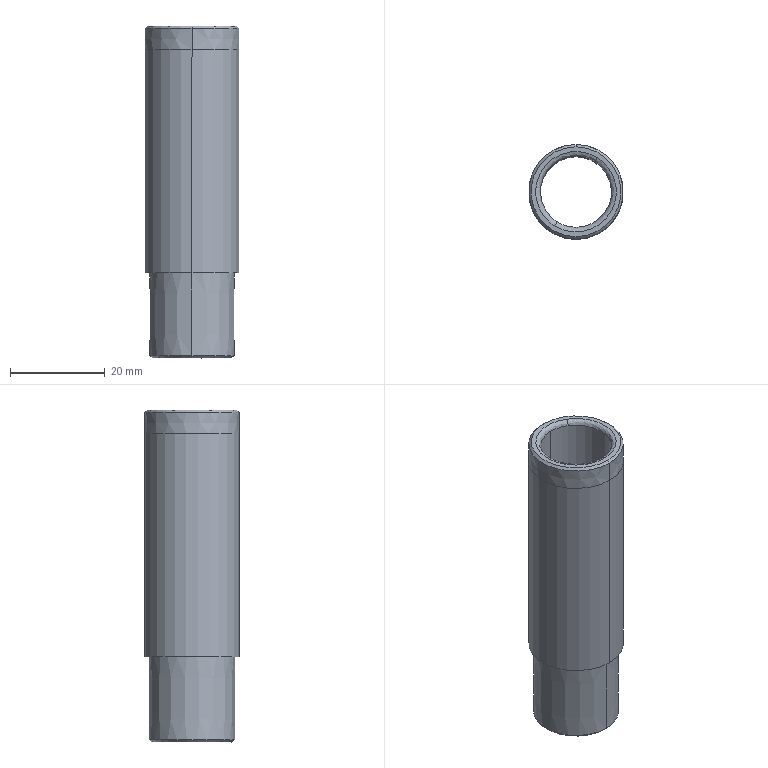Part | SolidWorks | features BaseBody 1 | 1 solid | 19 faces | box 20 x 20 x 70.171 mm | volume 8540 mm3 | cone 8 | spline 4 | cylinder 4 | plane 3 | commonest cylinder face diameters 15 x2 20 x2
STEP:
#1=CARTESIAN_POINT('',(700.535,31.172,-70.73));
#2=VERTEX_POINT('',#1);
#3=CARTESIAN_POINT('',(704.511,45.031,-70.73));
#4=VERTEX_POINT('',#3);
#5=CARTESIAN_POINT('',(700.535,38.672,-70.73));
#6=DIRECTION('',(0.000000001,-0.000000003,1.));
#7=DIRECTION('',(0.,-1.,-0.000000003));
#8=AXIS2_PLACEMENT_3D('',#5,#6,#7);
#9=CIRCLE('',#8,7.5);
#10=EDGE_CURVE('',#2,#4,#9,.T.);
#11=ORIENTED_EDGE('',*,*,#10,.T.);
#12=CARTESIAN_POINT('',(704.776,45.455,-71.23));
#13=VERTEX_POINT('',#12);
#14=CARTESIAN_POINT('',(704.776,45.455,-70.73));
#15=DIRECTION('',(0.8479,-0.5302,-0.000000002));
#16=DIRECTION('',(0.5302,0.8479,0.000000002));
#17=AXIS2_PLACEMENT_3D('',#14,#15,#16);
#18=CIRCLE('',#17,0.5);
#19=EDGE_CURVE('',#4,#13,#18,.T.);
#20=ORIENTED_EDGE('',*,*,#19,.T.);
#21=CARTESIAN_POINT('',(696.293,31.889,-71.23));
#22=VERTEX_POINT('',#21);
#23=CARTESIAN_POINT('',(704.776,45.455,-71.23));
#24=CARTESIAN_POINT('',(718.342,36.972,-71.23));
#25=CARTESIAN_POINT('',(709.86,23.406,-71.23));
#26=CARTESIAN_POINT('',(696.293,31.889,-71.23));
#27=(BOUNDED_CURVE()B_SPLINE_CURVE(3,(#23,#24,#25,#26),.UNSPECIFIED.,.F.,.F.)B_SPLINE_CURVE_WITH_KNOTS((4,4),(0.,1.),.UNSPECIFIED.)CURVE()GEOMETRIC_REPRESENTATION_ITEM()RATIONAL_B_SPLINE_CURVE((1.,0.3333,0.3333,1.))REPRESENTATION_ITEM(''));
#28=EDGE_CURVE('',#13,#22,#27,.T.);
#29=ORIENTED_EDGE('',*,*,#28,.T.);
#30=CARTESIAN_POINT('',(696.558,32.313,-70.73));
#31=VERTEX_POINT('',#30);
#32=CARTESIAN_POINT('',(696.293,31.889,-70.73));
#33=DIRECTION('',(-0.8479,0.5302,0.000000002));
#34=DIRECTION('',(-0.5302,-0.8479,-0.000000002));
#35=AXIS2_PLACEMENT_3D('',#32,#33,#34);
#36=CIRCLE('',#35,0.5);
#37=EDGE_CURVE('',#31,#22,#36,.T.);
#38=ORIENTED_EDGE('',*,*,#37,.F.);
#39=CARTESIAN_POINT('',(700.535,38.672,-70.73));
#40=DIRECTION('',(0.000000001,-0.000000003,1.));
#41=DIRECTION('',(0.,-1.,-0.000000003));
#42=AXIS2_PLACEMENT_3D('',#39,#40,#41);
#43=CIRCLE('',#42,7.5);
#44=EDGE_CURVE('',#31,#2,#43,.T.);
#45=ORIENTED_EDGE('',*,*,#44,.T.);
#46=EDGE_LOOP('',(#11,#20,#29,#38,#45));
#47=FACE_OUTER_BOUND('',#46,.T.);
#48=CARTESIAN_POINT('',(704.511,45.031,-70.73));
#49=CARTESIAN_POINT('',(717.229,37.079,-70.73));
#50=CARTESIAN_POINT('',(709.277,24.36,-70.73));
#51=CARTESIAN_POINT('',(696.558,32.313,-70.73));
#52=CARTESIAN_POINT('',(704.511,45.031,-71.023));
#53=CARTESIAN_POINT('',(717.229,37.079,-71.023));
#54=CARTESIAN_POINT('',(709.277,24.36,-71.023));
#55=CARTESIAN_POINT('',(696.558,32.313,-71.023));
#56=CARTESIAN_POINT('',(704.621,45.207,-71.23));
#57=CARTESIAN_POINT('',(717.69,37.035,-71.23));
#58=CARTESIAN_POINT('',(709.518,23.965,-71.23));
#59=CARTESIAN_POINT('',(696.449,32.137,-71.23));
#60=CARTESIAN_POINT('',(704.776,45.455,-71.23));
#61=CARTESIAN_POINT('',(718.342,36.972,-71.23));
#62=CARTESIAN_POINT('',(709.86,23.406,-71.23));
#63=CARTESIAN_POINT('',(696.293,31.889,-71.23));
#64=(BOUNDED_SURFACE()B_SPLINE_SURFACE(3,3,((#48,#49,#50,#51),(#52,#53,#54,#55),(#56,#57,#58,#59),(#60,#61,#62,#63)),.UNSPECIFIED.,.F.,.F.,.F.)B_SPLINE_SURFACE_WITH_KNOTS((4,4),(4,4),(0.,1.),(0.,1.),.UNSPECIFIED.)GEOMETRIC_REPRESENTATION_ITEM()RATIONAL_B_SPLINE_SURFACE(((1.,0.3333,0.3333,1.),(0.8047,0.2682,0.2682,0.8047),(0.8047,0.2682,0.2682,0.8047),(1.,0.3333,0.3333,1.)))REPRESENTATION_ITEM('')SURFACE());
#65=ADVANCED_FACE('',(#47),#64,.T.);
#66=CARTESIAN_POINT('',(700.535,31.172,-2.059));
#67=VERTEX_POINT('',#66);
#68=CARTESIAN_POINT('',(696.558,32.313,-2.059));
#69=VERTEX_POINT('',#68);
#70=CARTESIAN_POINT('',(700.535,38.672,-2.059));
#71=DIRECTION('',(-0.000000001,0.000000003,-1.));
#72=DIRECTION('',(0.,-1.,-0.000000003));
#73=AXIS2_PLACEMENT_3D('',#70,#71,#72);
#74=CIRCLE('',#73,7.5);
#75=EDGE_CURVE('',#67,#69,#74,.T.);
#76=ORIENTED_EDGE('',*,*,#75,.T.);
#77=CARTESIAN_POINT('',(696.028,31.465,-1.059));
#78=VERTEX_POINT('',#77);
#79=CARTESIAN_POINT('',(696.028,31.465,-2.059));
#80=DIRECTION('',(0.8479,-0.5302,-0.000000002));
#81=DIRECTION('',(-0.5302,-0.8479,-0.000000002));
#82=AXIS2_PLACEMENT_3D('',#79,#80,#81);
#83=CIRCLE('',#82,1.);
#84=EDGE_CURVE('',#69,#78,#83,.T.);
#85=ORIENTED_EDGE('',*,*,#84,.T.);
#86=CARTESIAN_POINT('',(705.041,45.879,-1.059));
#87=VERTEX_POINT('',#86);
#88=CARTESIAN_POINT('',(696.028,31.465,-1.059));
#89=CARTESIAN_POINT('',(710.442,22.452,-1.059));
#90=CARTESIAN_POINT('',(719.455,36.866,-1.059));
#91=CARTESIAN_POINT('',(705.041,45.879,-1.059));
#92=(BOUNDED_CURVE()B_SPLINE_CURVE(3,(#88,#89,#90,#91),.UNSPECIFIED.,.F.,.F.)B_SPLINE_CURVE_WITH_KNOTS((4,4),(0.,1.),.UNSPECIFIED.)CURVE()GEOMETRIC_REPRESENTATION_ITEM()RATIONAL_B_SPLINE_CURVE((1.,0.3333,0.3333,1.))REPRESENTATION_ITEM(''));
#93=EDGE_CURVE('',#78,#87,#92,.T.);
#94=ORIENTED_EDGE('',*,*,#93,.T.);
#95=CARTESIAN_POINT('',(704.511,45.031,-2.059));
#96=VERTEX_POINT('',#95);
#97=CARTESIAN_POINT('',(705.041,45.879,-2.059));
#98=DIRECTION('',(-0.8479,0.5302,0.000000002));
#99=DIRECTION('',(0.5302,0.8479,0.000000002));
#100=AXIS2_PLACEMENT_3D('',#97,#98,#99);
#101=CIRCLE('',#100,1.);
#102=EDGE_CURVE('',#96,#87,#101,.T.);
#103=ORIENTED_EDGE('',*,*,#102,.F.);
#104=CARTESIAN_POINT('',(700.535,38.672,-2.059));
#105=DIRECTION('',(-0.000000001,0.000000003,-1.));
#106=DIRECTION('',(0.,-1.,-0.000000003));
#107=AXIS2_PLACEMENT_3D('',#104,#105,#106);
#108=CIRCLE('',#107,7.5);
#109=EDGE_CURVE('',#96,#67,#108,.T.);
#110=ORIENTED_EDGE('',*,*,#109,.T.);
#111=EDGE_LOOP('',(#76,#85,#94,#103,#110));
#112=FACE_OUTER_BOUND('',#111,.T.);
#113=CARTESIAN_POINT('',(696.558,32.313,-2.059));
#114=CARTESIAN_POINT('',(709.277,24.36,-2.059));
#115=CARTESIAN_POINT('',(717.229,37.079,-2.059));
#116=CARTESIAN_POINT('',(704.511,45.031,-2.059));
#117=CARTESIAN_POINT('',(696.558,32.313,-1.473));
#118=CARTESIAN_POINT('',(709.277,24.36,-1.473));
#119=CARTESIAN_POINT('',(717.229,37.079,-1.473));
#120=CARTESIAN_POINT('',(704.511,45.031,-1.473));
#121=CARTESIAN_POINT('',(696.339,31.962,-1.059));
#122=CARTESIAN_POINT('',(709.76,23.57,-1.059));
#123=CARTESIAN_POINT('',(718.151,36.991,-1.059));
#124=CARTESIAN_POINT('',(704.731,45.383,-1.059));
#125=CARTESIAN_POINT('',(696.028,31.465,-1.059));
#126=CARTESIAN_POINT('',(710.442,22.452,-1.059));
#127=CARTESIAN_POINT('',(719.455,36.866,-1.059));
#128=CARTESIAN_POINT('',(705.041,45.879,-1.059));
#129=(BOUNDED_SURFACE()B_SPLINE_SURFACE(3,3,((#113,#114,#115,#116),(#117,#118,#119,#120),(#121,#122,#123,#124),(#125,#126,#127,#128)),.UNSPECIFIED.,.F.,.F.,.F.)B_SPLINE_SURFACE_WITH_KNOTS((4,4),(4,4),(0.,1.),(0.,1.),.UNSPECIFIED.)GEOMETRIC_REPRESENTATION_ITEM()RATIONAL_B_SPLINE_SURFACE(((1.,0.3333,0.3333,1.),(0.8047,0.2682,0.2682,0.8047),(0.8047,0.2682,0.2682,0.8047),(1.,0.3333,0.3333,1.)))REPRESENTATION_ITEM('')SURFACE());
#130=ADVANCED_FACE('',(#112),#129,.T.);
#131=CARTESIAN_POINT('',(700.535,46.172,-70.73));
#132=VERTEX_POINT('',#131);
#133=CARTESIAN_POINT('',(700.535,38.672,-70.73));
#134=DIRECTION('',(0.000000001,-0.000000003,1.));
#135=DIRECTION('',(0.,-1.,-0.000000003));
#136=AXIS2_PLACEMENT_3D('',#133,#134,#135);
#137=CIRCLE('',#136,7.5);
#138=EDGE_CURVE('',#132,#31,#137,.T.);
#139=ORIENTED_EDGE('',*,*,#138,.F.);
#140=CARTESIAN_POINT('',(700.535,46.172,-2.059));
#141=VERTEX_POINT('',#140);
#142=CARTESIAN_POINT('',(700.535,46.172,-1.059));
#143=DIRECTION('',(0.000000001,-0.000000003,1.));
#144=VECTOR('',#143,1000.);
#145=LINE('',#142,#144);
#146=EDGE_CURVE('',#132,#141,#145,.T.);
#147=ORIENTED_EDGE('',*,*,#146,.T.);
#148=CARTESIAN_POINT('',(700.535,38.672,-2.059));
#149=DIRECTION('',(-0.000000001,0.000000003,-1.));
#150=DIRECTION('',(0.,-1.,-0.000000003));
#151=AXIS2_PLACEMENT_3D('',#148,#149,#150);
#152=CIRCLE('',#151,7.5);
#153=EDGE_CURVE('',#69,#141,#152,.T.);
#154=ORIENTED_EDGE('',*,*,#153,.F.);
#155=ORIENTED_EDGE('',*,*,#75,.F.);
#156=CARTESIAN_POINT('',(700.535,31.172,-1.059));
#157=DIRECTION('',(0.000000001,-0.000000003,1.));
#158=VECTOR('',#157,1000.);
#159=LINE('',#156,#158);
#160=EDGE_CURVE('',#2,#67,#159,.T.);
#161=ORIENTED_EDGE('',*,*,#160,.F.);
#162=ORIENTED_EDGE('',*,*,#44,.F.);
#163=EDGE_LOOP('',(#139,#147,#154,#155,#161,#162));
#164=FACE_OUTER_BOUND('',#163,.T.);
#165=CARTESIAN_POINT('',(700.535,38.672,-1.059));
#166=DIRECTION('',(0.000000001,-0.000000003,1.));
#167=DIRECTION('',(0.,-1.,-0.000000003));
#168=AXIS2_PLACEMENT_3D('',#165,#166,#167);
#169=CYLINDRICAL_SURFACE('',#168,7.5);
#170=ADVANCED_FACE('',(#164),#169,.F.);
#171=CARTESIAN_POINT('',(700.535,47.169,-71.23));
#172=VERTEX_POINT('',#171);
#173=CARTESIAN_POINT('',(700.535,30.175,-71.23));
#174=VERTEX_POINT('',#173);
#175=CARTESIAN_POINT('',(700.535,38.672,-71.23));
#176=DIRECTION('',(-0.000000001,0.000000003,-1.));
#177=DIRECTION('',(0.,-1.,-0.000000003));
#178=AXIS2_PLACEMENT_3D('',#175,#176,#177);
#179=CIRCLE('',#178,8.497);
#180=EDGE_CURVE('',#172,#174,#179,.T.);
#181=ORIENTED_EDGE('',*,*,#180,.F.);
#182=CARTESIAN_POINT('',(700.535,47.669,-70.73));
#183=VERTEX_POINT('',#182);
#184=CARTESIAN_POINT('',(700.535,47.669,-70.73));
#185=DIRECTION('',(0.000000001,0.7072,0.707));
#186=VECTOR('',#185,1000.);
#187=LINE('',#184,#186);
#188=EDGE_CURVE('',#172,#183,#187,.T.);
#189=ORIENTED_EDGE('',*,*,#188,.T.);
#190=CARTESIAN_POINT('',(700.535,29.675,-70.73));
#191=VERTEX_POINT('',#190);
#192=CARTESIAN_POINT('',(700.535,38.672,-70.73));
#193=DIRECTION('',(-0.000000001,0.000000003,-1.));
#194=DIRECTION('',(0.5302,0.8479,0.000000002));
#195=AXIS2_PLACEMENT_3D('',#192,#193,#194);
#196=CIRCLE('',#195,8.997);
#197=EDGE_CURVE('',#183,#191,#196,.T.);
#198=ORIENTED_EDGE('',*,*,#197,.T.);
#199=CARTESIAN_POINT('',(700.535,29.675,-70.73));
#200=DIRECTION('',(0.000000001,-0.7072,0.707));
#201=VECTOR('',#200,1000.);
#202=LINE('',#199,#201);
#203=EDGE_CURVE('',#174,#191,#202,.T.);
#204=ORIENTED_EDGE('',*,*,#203,.F.);
#205=EDGE_LOOP('',(#181,#189,#198,#204));
#206=FACE_OUTER_BOUND('',#205,.T.);
#207=CARTESIAN_POINT('',(700.535,38.672,-70.73));
#208=DIRECTION('',(0.000000001,-0.000000003,1.));
#209=DIRECTION('',(0.,-1.,-0.000000003));
#210=AXIS2_PLACEMENT_3D('',#207,#208,#209);
#211=CONICAL_SURFACE('',#210,8.997,0.7855);
#212=ADVANCED_FACE('',(#206),#211,.T.);
#213=CARTESIAN_POINT('',(700.535,29.173,-1.059));
#214=VERTEX_POINT('',#213);
#215=CARTESIAN_POINT('',(700.535,48.171,-1.059));
#216=VERTEX_POINT('',#215);
#217=CARTESIAN_POINT('',(700.535,38.672,-1.059));
#218=DIRECTION('',(0.000000001,-0.000000003,1.));
#219=DIRECTION('',(0.,1.,0.000000003));
#220=AXIS2_PLACEMENT_3D('',#217,#218,#219);
#221=CIRCLE('',#220,9.499);
#222=EDGE_CURVE('',#214,#216,#221,.T.);
#223=ORIENTED_EDGE('',*,*,#222,.F.);
#224=CARTESIAN_POINT('',(700.535,28.673,-1.559));
#225=VERTEX_POINT('',#224);
#226=CARTESIAN_POINT('',(700.535,28.673,-1.559));
#227=DIRECTION('',(-0.000000001,-0.7072,-0.707));
#228=VECTOR('',#227,1000.);
#229=LINE('',#226,#228);
#230=EDGE_CURVE('',#214,#225,#229,.T.);
#231=ORIENTED_EDGE('',*,*,#230,.T.);
#232=CARTESIAN_POINT('',(700.535,48.671,-1.559));
#233=VERTEX_POINT('',#232);
#234=CARTESIAN_POINT('',(700.535,38.672,-1.559));
#235=DIRECTION('',(0.000000001,-0.000000003,1.));
#236=DIRECTION('',(0.5302,0.8479,0.000000002));
#237=AXIS2_PLACEMENT_3D('',#234,#235,#236);
#238=CIRCLE('',#237,9.999);
#239=EDGE_CURVE('',#225,#233,#238,.T.);
#240=ORIENTED_EDGE('',*,*,#239,.T.);
#241=CARTESIAN_POINT('',(700.535,48.671,-1.559));
#242=DIRECTION('',(-0.000000001,0.7072,-0.707));
#243=VECTOR('',#242,1000.);
#244=LINE('',#241,#243);
#245=EDGE_CURVE('',#216,#233,#244,.T.);
#246=ORIENTED_EDGE('',*,*,#245,.F.);
#247=EDGE_LOOP('',(#223,#231,#240,#246));
#248=FACE_OUTER_BOUND('',#247,.T.);
#249=CARTESIAN_POINT('',(700.535,38.672,-1.559));
#250=DIRECTION('',(-0.000000001,0.000000003,-1.));
#251=DIRECTION('',(0.,1.,0.000000003));
#252=AXIS2_PLACEMENT_3D('',#249,#250,#251);
#253=CONICAL_SURFACE('',#252,9.999,0.7855);
#254=ADVANCED_FACE('',(#248),#253,.T.);
#255=ORIENTED_EDGE('',*,*,#197,.F.);
#256=CARTESIAN_POINT('',(700.535,47.672,-53.23));
#257=VERTEX_POINT('',#256);
#258=CARTESIAN_POINT('',(700.535,47.672,-53.23));
#259=DIRECTION('',(0.000000001,0.0001745,1.));
#260=VECTOR('',#259,1000.);
#261=LINE('',#258,#260);
#262=EDGE_CURVE('',#183,#257,#261,.T.);
#263=ORIENTED_EDGE('',*,*,#262,.T.);
#264=CARTESIAN_POINT('',(700.535,29.672,-53.23));
#265=VERTEX_POINT('',#264);
#266=CARTESIAN_POINT('',(700.535,38.672,-53.23));
#267=DIRECTION('',(-0.000000001,0.000000003,-1.));
#268=DIRECTION('',(0.,-1.,-0.000000003));
#269=AXIS2_PLACEMENT_3D('',#266,#267,#268);
#270=CIRCLE('',#269,9.);
#271=EDGE_CURVE('',#257,#265,#270,.T.);
#272=ORIENTED_EDGE('',*,*,#271,.T.);
#273=CARTESIAN_POINT('',(700.535,29.672,-53.23));
#274=DIRECTION('',(0.000000001,-0.0001745,1.));
#275=VECTOR('',#274,1000.);
#276=LINE('',#273,#275);
#277=EDGE_CURVE('',#191,#265,#276,.T.);
#278=ORIENTED_EDGE('',*,*,#277,.F.);
#279=EDGE_LOOP('',(#255,#263,#272,#278));
#280=FACE_OUTER_BOUND('',#279,.T.);
#281=CARTESIAN_POINT('',(700.535,38.672,-53.23));
#282=DIRECTION('',(0.000000001,-0.000000003,1.));
#283=DIRECTION('',(0.,-1.,-0.000000003));
#284=AXIS2_PLACEMENT_3D('',#281,#282,#283);
#285=CONICAL_SURFACE('',#284,9.,0.0001745);
#286=ADVANCED_FACE('',(#280),#285,.T.);
#287=ORIENTED_EDGE('',*,*,#239,.F.);
#288=CARTESIAN_POINT('',(700.535,28.672,-6.059));
#289=VERTEX_POINT('',#288);
#290=CARTESIAN_POINT('',(700.535,28.672,-6.059));
#291=DIRECTION('',(-0.000000001,-0.0001745,-1.));
#292=VECTOR('',#291,1000.);
#293=LINE('',#290,#292);
#294=EDGE_CURVE('',#225,#289,#293,.T.);
#295=ORIENTED_EDGE('',*,*,#294,.T.);
#296=CARTESIAN_POINT('',(700.535,48.672,-6.059));
#297=VERTEX_POINT('',#296);
#298=CARTESIAN_POINT('',(700.535,38.672,-6.059));
#299=DIRECTION('',(0.000000001,-0.000000003,1.));
#300=DIRECTION('',(-0.5302,-0.8479,-0.000000002));
#301=AXIS2_PLACEMENT_3D('',#298,#299,#300);
#302=CIRCLE('',#301,10.);
#303=EDGE_CURVE('',#289,#297,#302,.T.);
#304=ORIENTED_EDGE('',*,*,#303,.T.);
#305=CARTESIAN_POINT('',(700.535,48.672,-6.059));
#306=DIRECTION('',(-0.000000001,0.0001745,-1.));
#307=VECTOR('',#306,1000.);
#308=LINE('',#305,#307);
#309=EDGE_CURVE('',#233,#297,#308,.T.);
#310=ORIENTED_EDGE('',*,*,#309,.F.);
#311=EDGE_LOOP('',(#287,#295,#304,#310));
#312=FACE_OUTER_BOUND('',#311,.T.);
#313=CARTESIAN_POINT('',(700.535,38.672,-6.059));
#314=DIRECTION('',(-0.000000001,0.000000003,-1.));
#315=DIRECTION('',(0.,1.,0.000000003));
#316=AXIS2_PLACEMENT_3D('',#313,#314,#315);
#317=CONICAL_SURFACE('',#316,10.,0.0001745);
#318=ADVANCED_FACE('',(#312),#317,.T.);
#319=CARTESIAN_POINT('',(700.535,48.672,-53.23));
#320=VERTEX_POINT('',#319);
#321=CARTESIAN_POINT('',(700.535,28.672,-53.23));
#322=VERTEX_POINT('',#321);
#323=CARTESIAN_POINT('',(700.535,38.672,-53.23));
#324=DIRECTION('',(-0.000000001,0.000000003,-1.));
#325=DIRECTION('',(0.,-1.,-0.000000003));
#326=AXIS2_PLACEMENT_3D('',#323,#324,#325);
#327=CIRCLE('',#326,10.);
#328=EDGE_CURVE('',#320,#322,#327,.T.);
#329=ORIENTED_EDGE('',*,*,#328,.F.);
#330=CARTESIAN_POINT('',(700.535,48.672,-6.059));
#331=DIRECTION('',(0.000000001,-0.000000003,1.));
#332=VECTOR('',#331,1000.);
#333=LINE('',#330,#332);
#334=EDGE_CURVE('',#320,#297,#333,.T.);
#335=ORIENTED_EDGE('',*,*,#334,.T.);
#336=ORIENTED_EDGE('',*,*,#303,.F.);
#337=CARTESIAN_POINT('',(700.535,28.672,-6.059));
#338=DIRECTION('',(0.000000001,-0.000000003,1.));
#339=VECTOR('',#338,1000.);
#340=LINE('',#337,#339);
#341=EDGE_CURVE('',#322,#289,#340,.T.);
#342=ORIENTED_EDGE('',*,*,#341,.F.);
#343=EDGE_LOOP('',(#329,#335,#336,#342));
#344=FACE_OUTER_BOUND('',#343,.T.);
#345=CARTESIAN_POINT('',(700.535,38.672,-6.059));
#346=DIRECTION('',(0.000000001,-0.000000003,1.));
#347=DIRECTION('',(0.,-1.,-0.000000003));
#348=AXIS2_PLACEMENT_3D('',#345,#346,#347);
#349=CYLINDRICAL_SURFACE('',#348,10.);
#350=ADVANCED_FACE('',(#344),#349,.T.);
#351=ORIENTED_EDGE('',*,*,#146,.F.);
#352=CARTESIAN_POINT('',(700.535,38.672,-70.73));
#353=DIRECTION('',(0.000000001,-0.000000003,1.));
#354=DIRECTION('',(0.,-1.,-0.000000003));
#355=AXIS2_PLACEMENT_3D('',#352,#353,#354);
#356=CIRCLE('',#355,7.5);
#357=EDGE_CURVE('',#4,#132,#356,.T.);
#358=ORIENTED_EDGE('',*,*,#357,.F.);
#359=ORIENTED_EDGE('',*,*,#10,.F.);
#360=ORIENTED_EDGE('',*,*,#160,.T.);
#361=ORIENTED_EDGE('',*,*,#109,.F.);
#362=CARTESIAN_POINT('',(700.535,38.672,-2.059));
#363=DIRECTION('',(-0.000000001,0.000000003,-1.));
#364=DIRECTION('',(0.,-1.,-0.000000003));
#365=AXIS2_PLACEMENT_3D('',#362,#363,#364);
#366=CIRCLE('',#365,7.5);
#367=EDGE_CURVE('',#141,#96,#366,.T.);
#368=ORIENTED_EDGE('',*,*,#367,.F.);
#369=EDGE_LOOP('',(#351,#358,#359,#360,#361,#368));
#370=FACE_OUTER_BOUND('',#369,.T.);
#371=CARTESIAN_POINT('',(700.535,38.672,-1.059));
#372=DIRECTION('',(0.000000001,-0.000000003,1.));
#373=DIRECTION('',(0.,-1.,-0.000000003));
#374=AXIS2_PLACEMENT_3D('',#371,#372,#373);
#375=CYLINDRICAL_SURFACE('',#374,7.5);
#376=ADVANCED_FACE('',(#370),#375,.F.);
#377=ORIENTED_EDGE('',*,*,#19,.F.);
#378=ORIENTED_EDGE('',*,*,#357,.T.);
#379=ORIENTED_EDGE('',*,*,#138,.T.);
#380=ORIENTED_EDGE('',*,*,#37,.T.);
#381=CARTESIAN_POINT('',(696.293,31.889,-71.23));
#382=CARTESIAN_POINT('',(682.727,40.372,-71.23));
#383=CARTESIAN_POINT('',(691.21,53.938,-71.23));
#384=CARTESIAN_POINT('',(704.776,45.455,-71.23));
#385=(BOUNDED_CURVE()B_SPLINE_CURVE(3,(#381,#382,#383,#384),.UNSPECIFIED.,.F.,.F.)B_SPLINE_CURVE_WITH_KNOTS((4,4),(0.,1.),.UNSPECIFIED.)CURVE()GEOMETRIC_REPRESENTATION_ITEM()RATIONAL_B_SPLINE_CURVE((1.,0.3333,0.3333,1.))REPRESENTATION_ITEM(''));
#386=EDGE_CURVE('',#22,#13,#385,.T.);
#387=ORIENTED_EDGE('',*,*,#386,.T.);
#388=EDGE_LOOP('',(#377,#378,#379,#380,#387));
#389=FACE_OUTER_BOUND('',#388,.T.);
#390=CARTESIAN_POINT('',(696.558,32.313,-70.73));
#391=CARTESIAN_POINT('',(683.84,40.266,-70.73));
#392=CARTESIAN_POINT('',(691.793,52.984,-70.73));
#393=CARTESIAN_POINT('',(704.511,45.031,-70.73));
#394=CARTESIAN_POINT('',(696.558,32.313,-71.023));
#395=CARTESIAN_POINT('',(683.84,40.266,-71.023));
#396=CARTESIAN_POINT('',(691.793,52.984,-71.023));
#397=CARTESIAN_POINT('',(704.511,45.031,-71.023));
#398=CARTESIAN_POINT('',(696.449,32.137,-71.23));
#399=CARTESIAN_POINT('',(683.379,40.31,-71.23));
#400=CARTESIAN_POINT('',(691.551,53.379,-71.23));
#401=CARTESIAN_POINT('',(704.621,45.207,-71.23));
#402=CARTESIAN_POINT('',(696.293,31.889,-71.23));
#403=CARTESIAN_POINT('',(682.727,40.372,-71.23));
#404=CARTESIAN_POINT('',(691.21,53.938,-71.23));
#405=CARTESIAN_POINT('',(704.776,45.455,-71.23));
#406=(BOUNDED_SURFACE()B_SPLINE_SURFACE(3,3,((#390,#391,#392,#393),(#394,#395,#396,#397),(#398,#399,#400,#401),(#402,#403,#404,#405)),.UNSPECIFIED.,.F.,.F.,.T.)B_SPLINE_SURFACE_WITH_KNOTS((4,4),(4,4),(0.,1.),(0.,1.),.UNSPECIFIED.)GEOMETRIC_REPRESENTATION_ITEM()RATIONAL_B_SPLINE_SURFACE(((1.,0.3333,0.3333,1.),(0.8047,0.2682,0.2682,0.8047),(0.8047,0.2682,0.2682,0.8047),(1.,0.3333,0.3333,1.)))REPRESENTATION_ITEM('')SURFACE());
#407=ADVANCED_FACE('',(#389),#406,.T.);
#408=ORIENTED_EDGE('',*,*,#84,.F.);
#409=ORIENTED_EDGE('',*,*,#153,.T.);
#410=ORIENTED_EDGE('',*,*,#367,.T.);
#411=ORIENTED_EDGE('',*,*,#102,.T.);
#412=CARTESIAN_POINT('',(705.041,45.879,-1.059));
#413=CARTESIAN_POINT('',(690.627,54.892,-1.059));
#414=CARTESIAN_POINT('',(681.614,40.478,-1.059));
#415=CARTESIAN_POINT('',(696.028,31.465,-1.059));
#416=(BOUNDED_CURVE()B_SPLINE_CURVE(3,(#412,#413,#414,#415),.UNSPECIFIED.,.F.,.F.)B_SPLINE_CURVE_WITH_KNOTS((4,4),(0.,1.),.UNSPECIFIED.)CURVE()GEOMETRIC_REPRESENTATION_ITEM()RATIONAL_B_SPLINE_CURVE((1.,0.3333,0.3333,1.))REPRESENTATION_ITEM(''));
#417=EDGE_CURVE('',#87,#78,#416,.T.);
#418=ORIENTED_EDGE('',*,*,#417,.T.);
#419=EDGE_LOOP('',(#408,#409,#410,#411,#418));
#420=FACE_OUTER_BOUND('',#419,.T.);
#421=CARTESIAN_POINT('',(704.511,45.031,-2.059));
#422=CARTESIAN_POINT('',(691.793,52.984,-2.059));
#423=CARTESIAN_POINT('',(683.84,40.266,-2.059));
#424=CARTESIAN_POINT('',(696.558,32.313,-2.059));
#425=CARTESIAN_POINT('',(704.511,45.031,-1.473));
#426=CARTESIAN_POINT('',(691.793,52.984,-1.473));
#427=CARTESIAN_POINT('',(683.84,40.266,-1.473));
#428=CARTESIAN_POINT('',(696.558,32.313,-1.473));
#429=CARTESIAN_POINT('',(704.731,45.383,-1.059));
#430=CARTESIAN_POINT('',(691.31,53.774,-1.059));
#431=CARTESIAN_POINT('',(682.918,40.354,-1.059));
#432=CARTESIAN_POINT('',(696.339,31.962,-1.059));
#433=CARTESIAN_POINT('',(705.041,45.879,-1.059));
#434=CARTESIAN_POINT('',(690.627,54.892,-1.059));
#435=CARTESIAN_POINT('',(681.614,40.478,-1.059));
#436=CARTESIAN_POINT('',(696.028,31.465,-1.059));
#437=(BOUNDED_SURFACE()B_SPLINE_SURFACE(3,3,((#421,#422,#423,#424),(#425,#426,#427,#428),(#429,#430,#431,#432),(#433,#434,#435,#436)),.UNSPECIFIED.,.F.,.F.,.F.)B_SPLINE_SURFACE_WITH_KNOTS((4,4),(4,4),(0.,1.),(0.,1.),.UNSPECIFIED.)GEOMETRIC_REPRESENTATION_ITEM()RATIONAL_B_SPLINE_SURFACE(((1.,0.3333,0.3333,1.),(0.8047,0.2682,0.2682,0.8047),(0.8047,0.2682,0.2682,0.8047),(1.,0.3333,0.3333,1.)))REPRESENTATION_ITEM('')SURFACE());
#438=ADVANCED_FACE('',(#420),#437,.T.);
#439=ORIENTED_EDGE('',*,*,#28,.F.);
#440=ORIENTED_EDGE('',*,*,#386,.F.);
#441=EDGE_LOOP('',(#439,#440));
#442=FACE_BOUND('',#441,.T.);
#443=CARTESIAN_POINT('',(700.535,38.672,-71.23));
#444=DIRECTION('',(-0.000000001,0.000000003,-1.));
#445=DIRECTION('',(0.,-1.,-0.000000003));
#446=AXIS2_PLACEMENT_3D('',#443,#444,#445);
#447=CIRCLE('',#446,8.497);
#448=EDGE_CURVE('',#174,#172,#447,.T.);
#449=ORIENTED_EDGE('',*,*,#448,.T.);
#450=ORIENTED_EDGE('',*,*,#180,.T.);
#451=EDGE_LOOP('',(#449,#450));
#452=FACE_OUTER_BOUND('',#451,.T.);
#453=CARTESIAN_POINT('',(700.535,38.672,-71.23));
#454=DIRECTION('',(-0.000000001,0.000000003,-1.));
#455=DIRECTION('',(0.,1.,0.000000003));
#456=AXIS2_PLACEMENT_3D('',#453,#454,#455);
#457=PLANE('',#456);
#458=ADVANCED_FACE('',(#442,#452),#457,.T.);
#459=ORIENTED_EDGE('',*,*,#93,.F.);
#460=ORIENTED_EDGE('',*,*,#417,.F.);
#461=EDGE_LOOP('',(#459,#460));
#462=FACE_BOUND('',#461,.T.);
#463=CARTESIAN_POINT('',(700.535,38.672,-1.059));
#464=DIRECTION('',(0.000000001,-0.000000003,1.));
#465=DIRECTION('',(0.,1.,0.000000003));
#466=AXIS2_PLACEMENT_3D('',#463,#464,#465);
#467=CIRCLE('',#466,9.499);
#468=EDGE_CURVE('',#216,#214,#467,.T.);
#469=ORIENTED_EDGE('',*,*,#468,.T.);
#470=ORIENTED_EDGE('',*,*,#222,.T.);
#471=EDGE_LOOP('',(#469,#470));
#472=FACE_OUTER_BOUND('',#471,.T.);
#473=CARTESIAN_POINT('',(700.535,38.672,-1.059));
#474=DIRECTION('',(0.000000001,-0.000000003,1.));
#475=DIRECTION('',(0.,-1.,-0.000000003));
#476=AXIS2_PLACEMENT_3D('',#473,#474,#475);
#477=PLANE('',#476);
#478=ADVANCED_FACE('',(#462,#472),#477,.T.);
#479=ORIENTED_EDGE('',*,*,#188,.F.);
#480=ORIENTED_EDGE('',*,*,#448,.F.);
#481=ORIENTED_EDGE('',*,*,#203,.T.);
#482=CARTESIAN_POINT('',(700.535,38.672,-70.73));
#483=DIRECTION('',(-0.000000001,0.000000003,-1.));
#484=DIRECTION('',(0.5302,0.8479,0.000000002));
#485=AXIS2_PLACEMENT_3D('',#482,#483,#484);
#486=CIRCLE('',#485,8.997);
#487=EDGE_CURVE('',#191,#183,#486,.T.);
#488=ORIENTED_EDGE('',*,*,#487,.T.);
#489=EDGE_LOOP('',(#479,#480,#481,#488));
#490=FACE_OUTER_BOUND('',#489,.T.);
#491=CARTESIAN_POINT('',(700.535,38.672,-70.73));
#492=DIRECTION('',(0.000000001,-0.000000003,1.));
#493=DIRECTION('',(0.,-1.,-0.000000003));
#494=AXIS2_PLACEMENT_3D('',#491,#492,#493);
#495=CONICAL_SURFACE('',#494,8.997,0.7855);
#496=ADVANCED_FACE('',(#490),#495,.T.);
#497=ORIENTED_EDGE('',*,*,#230,.F.);
#498=ORIENTED_EDGE('',*,*,#468,.F.);
#499=ORIENTED_EDGE('',*,*,#245,.T.);
#500=CARTESIAN_POINT('',(700.535,38.672,-1.559));
#501=DIRECTION('',(0.000000001,-0.000000003,1.));
#502=DIRECTION('',(0.5302,0.8479,0.000000002));
#503=AXIS2_PLACEMENT_3D('',#500,#501,#502);
#504=CIRCLE('',#503,9.999);
#505=EDGE_CURVE('',#233,#225,#504,.T.);
#506=ORIENTED_EDGE('',*,*,#505,.T.);
#507=EDGE_LOOP('',(#497,#498,#499,#506));
#508=FACE_OUTER_BOUND('',#507,.T.);
#509=CARTESIAN_POINT('',(700.535,38.672,-1.559));
#510=DIRECTION('',(-0.000000001,0.000000003,-1.));
#511=DIRECTION('',(0.,1.,0.000000003));
#512=AXIS2_PLACEMENT_3D('',#509,#510,#511);
#513=CONICAL_SURFACE('',#512,9.999,0.7855);
#514=ADVANCED_FACE('',(#508),#513,.T.);
#515=ORIENTED_EDGE('',*,*,#262,.F.);
#516=ORIENTED_EDGE('',*,*,#487,.F.);
#517=ORIENTED_EDGE('',*,*,#277,.T.);
#518=CARTESIAN_POINT('',(700.535,38.672,-53.23));
#519=DIRECTION('',(-0.000000001,0.000000003,-1.));
#520=DIRECTION('',(0.,-1.,-0.000000003));
#521=AXIS2_PLACEMENT_3D('',#518,#519,#520);
#522=CIRCLE('',#521,9.);
#523=EDGE_CURVE('',#265,#257,#522,.T.);
#524=ORIENTED_EDGE('',*,*,#523,.T.);
#525=EDGE_LOOP('',(#515,#516,#517,#524));
#526=FACE_OUTER_BOUND('',#525,.T.);
#527=CARTESIAN_POINT('',(700.535,38.672,-53.23));
#528=DIRECTION('',(0.000000001,-0.000000003,1.));
#529=DIRECTION('',(0.,-1.,-0.000000003));
#530=AXIS2_PLACEMENT_3D('',#527,#528,#529);
#531=CONICAL_SURFACE('',#530,9.,0.0001745);
#532=ADVANCED_FACE('',(#526),#531,.T.);
#533=ORIENTED_EDGE('',*,*,#294,.F.);
#534=ORIENTED_EDGE('',*,*,#505,.F.);
#535=ORIENTED_EDGE('',*,*,#309,.T.);
#536=CARTESIAN_POINT('',(700.535,38.672,-6.059));
#537=DIRECTION('',(0.000000001,-0.000000003,1.));
#538=DIRECTION('',(-0.5302,-0.8479,-0.000000002));
#539=AXIS2_PLACEMENT_3D('',#536,#537,#538);
#540=CIRCLE('',#539,10.);
#541=EDGE_CURVE('',#297,#289,#540,.T.);
#542=ORIENTED_EDGE('',*,*,#541,.T.);
#543=EDGE_LOOP('',(#533,#534,#535,#542));
#544=FACE_OUTER_BOUND('',#543,.T.);
#545=CARTESIAN_POINT('',(700.535,38.672,-6.059));
#546=DIRECTION('',(-0.000000001,0.000000003,-1.));
#547=DIRECTION('',(0.,1.,0.000000003));
#548=AXIS2_PLACEMENT_3D('',#545,#546,#547);
#549=CONICAL_SURFACE('',#548,10.,0.0001745);
#550=ADVANCED_FACE('',(#544),#549,.T.);
#551=CARTESIAN_POINT('',(700.535,38.672,-53.23));
#552=DIRECTION('',(-0.000000001,0.000000003,-1.));
#553=DIRECTION('',(0.,-1.,-0.000000003));
#554=AXIS2_PLACEMENT_3D('',#551,#552,#553);
#555=CIRCLE('',#554,10.);
#556=EDGE_CURVE('',#322,#320,#555,.T.);
#557=ORIENTED_EDGE('',*,*,#556,.T.);
#558=ORIENTED_EDGE('',*,*,#328,.T.);
#559=EDGE_LOOP('',(#557,#558));
#560=FACE_OUTER_BOUND('',#559,.T.);
#561=ORIENTED_EDGE('',*,*,#523,.F.);
#562=ORIENTED_EDGE('',*,*,#271,.F.);
#563=EDGE_LOOP('',(#561,#562));
#564=FACE_BOUND('',#563,.T.);
#565=CARTESIAN_POINT('',(700.535,38.672,-53.23));
#566=DIRECTION('',(-0.000000001,0.000000003,-1.));
#567=DIRECTION('',(0.,1.,0.000000003));
#568=AXIS2_PLACEMENT_3D('',#565,#566,#567);
#569=PLANE('',#568);
#570=ADVANCED_FACE('',(#560,#564),#569,.T.);
#571=ORIENTED_EDGE('',*,*,#334,.F.);
#572=ORIENTED_EDGE('',*,*,#556,.F.);
#573=ORIENTED_EDGE('',*,*,#341,.T.);
#574=ORIENTED_EDGE('',*,*,#541,.F.);
#575=EDGE_LOOP('',(#571,#572,#573,#574));
#576=FACE_OUTER_BOUND('',#575,.T.);
#577=CARTESIAN_POINT('',(700.535,38.672,-6.059));
#578=DIRECTION('',(0.000000001,-0.000000003,1.));
#579=DIRECTION('',(0.,-1.,-0.000000003));
#580=AXIS2_PLACEMENT_3D('',#577,#578,#579);
#581=CYLINDRICAL_SURFACE('',#580,10.);
#582=ADVANCED_FACE('',(#576),#581,.T.);
#583=CLOSED_SHELL('',(#65,#130,#170,#212,#254,#286,#318,#350,#376,#407,#438,#458,#478,#496,#514,#532,#550,#570,#582));
#584=MANIFOLD_SOLID_BREP('',#583);
#585=CARTESIAN_POINT('',(0.,0.,0.));
#586=DIRECTION('',(0.,0.,1.));
#587=DIRECTION('',(1.,0.,0.));
#588=AXIS2_PLACEMENT_3D('',#585,#586,#587);
#589=(LENGTH_UNIT()NAMED_UNIT(*)SI_UNIT(.MILLI.,.METRE.));
#590=UNCERTAINTY_MEASURE_WITH_UNIT(LENGTH_MEASURE(0.00001),#589,'','');
#591=(NAMED_UNIT(*)PLANE_ANGLE_UNIT()SI_UNIT($,.RADIAN.));
#592=(NAMED_UNIT(*)SI_UNIT($,.STERADIAN.)SOLID_ANGLE_UNIT());
#593=(GEOMETRIC_REPRESENTATION_CONTEXT(3)GLOBAL_UNCERTAINTY_ASSIGNED_CONTEXT((#590))GLOBAL_UNIT_ASSIGNED_CONTEXT((#589,#591,#592))REPRESENTATION_CONTEXT('',''));
#594=ADVANCED_BREP_SHAPE_REPRESENTATION('',(#584,#588),#593);